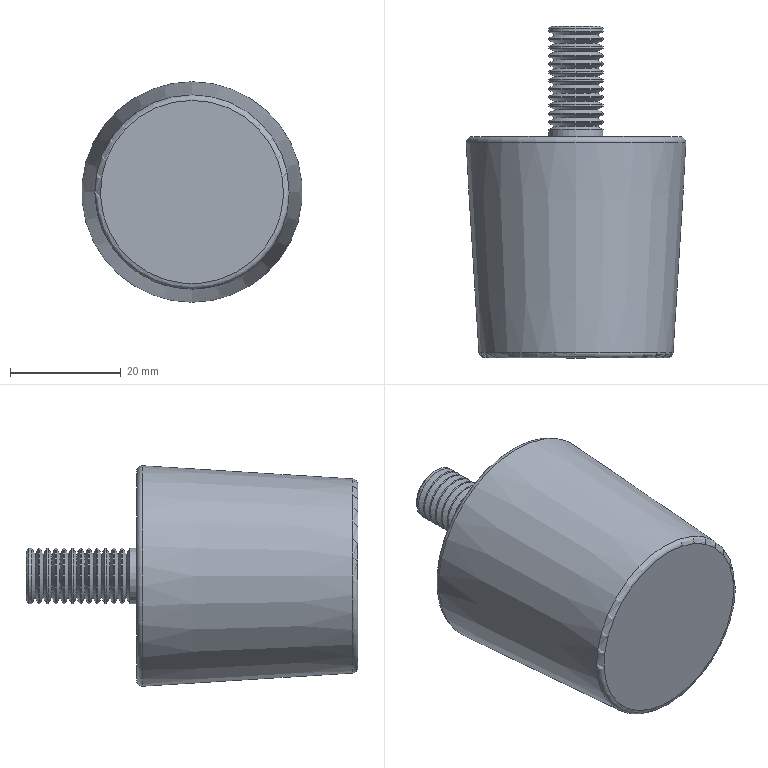Part | STEP file | 5090104W | 1 solid | 44 faces | box 39.871 x 60 x 39.871 mm | volume 45524 mm3 | cone 26 | cylinder 13 | plane 3 | torus 2 | commonest cylinder face diameters 10 x13